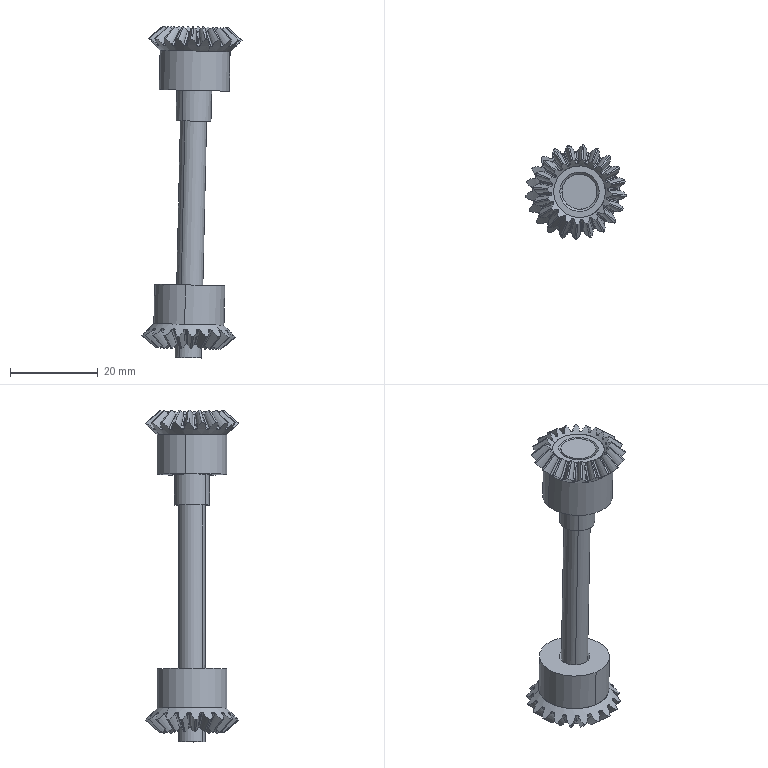Part | SolidWorks | 5 solids | 291 faces | box 22.911 x 21.375 x 75.748 mm | volume 7166 mm3 | spline 200 | cone 56 | cylinder 24 | plane 11 | commonest cylinder face diameters 11.8 x8 2.2 x4 6 x4 8 x4 16 x4